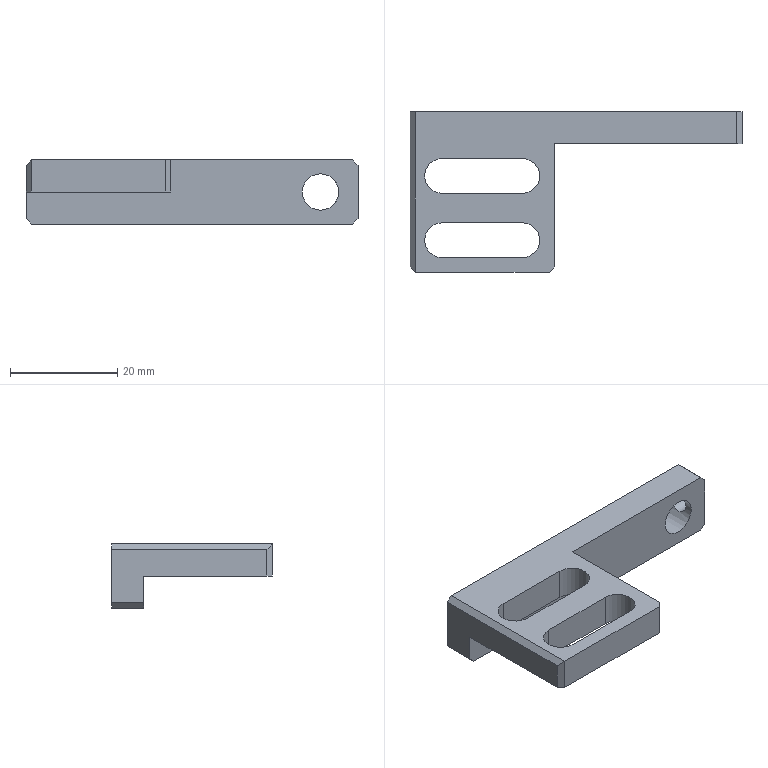NC program | NX | posted with a generic post | part box 62 x 30 x 12 mm
Lines 1 to 1127 of 2452:
N10 G17 G21 G94 G90
(FLOOR_WALL , TOOL : D80)
N12 T19 M6
N14 G54
N16 G17 G0 G90 X-79. Y0. S6500 M3
N18 G43 Z30. H19
N20 Z3.
N22 G94 G1 Z0. F1500.
N24 X-76.
N26 X76.
N28 X79.
N30 Z3.
N32 G0 Z30.
N34 M5
(ADAPTIVE_MILLING , TOOL : D10)
N36 T15 M6
N38 G54
N40 G17 G0 G90 X-43.696 Y9.051 S9500 M3
N42 G43 Z30. H15
N44 Z-9.
N46 G94 G1 Z-12. F1000.
N48 X-42.34 Y8.521 F3000.
N50 G3 X-41.05 Y9.051 R1.015
N52 X-40.406 Y12.21 R9.424
N54 X-40.205 Y17.805 R187.645
N56 G2 X-37.222 Y22.096 R6.12
N58 X-31.636 Y23.842 R13.446
N60 X-22.247 Y24.18 R89.73
N62 G1 X-20.347 Y24.185
N64 X-17.347 Y24.189
N66 X-10.147 Y24.19
N68 X33.353
N70 X33.453 Y24.188
N72 X33.553 Y24.183
N74 G2 X37.956 Y21.388 R5.941
N76 X39.823 Y15.744 R12.962
N78 X40.176 Y7.056 R79.199
N80 G1 X40.182 Y5.556
N82 X40.187 Y3.356
N84 X40.19 Y-0.444
N86 Y-17.344
N88 X40.189 Y-17.444
N90 X40.184 Y-17.544
N92 G2 X37.56 Y-21.836 R5.866
N94 X32.049 Y-23.779 R12.34
N96 X23.864 Y-24.17 R67.44
N98 G1 X22.564 Y-24.178
N100 X20.964 Y-24.184
N102 X18.464 Y-24.188
N104 X13.564 Y-24.19
N106 X-33.336
N108 X-33.436 Y-24.189
N110 G2 X-37.832 Y-21.568 R5.82
N112 X-39.764 Y-16.158 R12.207
N114 X-40.172 Y-7.474 R69.436
N116 X-40.159 Y6.625 R759.67
N118 G3 X-39.485 Y15.297 R155.91
N120 G2 X-35.334 Y21.202 R7.866
N122 X-28.936 Y23.024 R16.463
N124 X-19.346 Y23.367 R100.863
N126 G1 X-17.646 Y23.374
N128 X-15.246 Y23.378
N130 X-11.046 Y23.381
N132 X9.754 Y23.382
N134 X30.454
N136 X30.654 Y23.38
N138 G2 X36.983 Y19.6 R7.588
N140 X38.954 Y13.459 R15.207
N142 X39.366 Y3.573 R87.274
N144 G1 X39.373 Y1.873
N146 X39.378 Y-0.427
N148 X39.381 Y-4.227
N150 X39.382 Y-14.527
N152 X39.381 Y-14.627
N154 X39.376 Y-14.827
N156 G2 X35.623 Y-20.967 R7.581
N158 X29.584 Y-22.934 R14.985
N160 X20. Y-23.363 R80.802
N162 G1 X18.4 Y-23.371
N164 X16.4 Y-23.376
N166 X13.3 Y-23.38
N168 X6.2 Y-23.382
N170 X-30.5
N172 X-30.7 Y-23.38
N174 G2 X-36.954 Y-19.648 R7.559
N176 X-38.956 Y-13.414 R15.247
N178 X-39.361 Y-4.328 R81.183
N180 X-39.306 Y5.97 R217.252
N182 X-38.737 Y13.648 R271.341
N184 X-33.658 Y20.415 R9.134
N186 X-26.832 Y22.212 R18.952
N188 X-15.442 Y22.563 R126.701
N190 G1 X-13.242 Y22.568
N192 X-9.742 Y22.572
N194 X-1.242 Y22.573
N196 X28.158
N198 X28.358 Y22.571
N200 X28.558 Y22.567
N202 G2 X36.25 Y17.814 R8.78
N204 X38.166 Y11.129 R17.751
N206 X38.556 Y0.742 R103.678
N208 X38.545 Y-13.058 R767.731
N210 X33.726 Y-20.299 R8.807
N212 X27.028 Y-22.175 R18.02
N214 X16.939 Y-22.556 R103.246
N216 G1 X15.339 Y-22.563
N218 X13.039 Y-22.568
N220 X9.439 Y-22.572
N222 X0.139 Y-22.573
N224 X-28.161
N226 X-28.361 Y-22.571
N228 G2 X-36.299 Y-17.724 R8.819
N230 X-38.175 Y-11.027 R18.
N232 X-38.556 Y-0.938 R103.676
N234 X-38.023 Y11.943 R113.361
N236 X-35.561 Y17.211 R10.199
N238 X-32.473 Y19.87 R5.126
N240 X-23.965 Y21.514 R28.511
N242 X-11.069 Y21.759 R226.459
N244 G1 X-7.669 Y21.763
N246 X-0.269 Y21.764
N248 X26.131
N250 X26.331 Y21.763
N252 X26.531 Y21.76
N254 X26.731 Y21.755
N256 G2 X32.627 Y19.799 R9.712
N258 X34.648 Y18.552 R5.351
N260 X35.9 Y16.384 R5.818
N262 X37.518 Y7.868 R29.466
N264 X37.76 Y-5.528 R242.06
N266 X37.694 Y-11.726 R97.141
N268 X33.047 Y-19.035 R9.453
N270 X30.839 Y-20.166 R6.945
N272 X23.089 Y-21.543 R27.373
N274 X10.292 Y-21.76 R245.397
N276 G1 X6.292 Y-21.763
N278 X-5.208 Y-21.765
N280 X-26.108 Y-21.764
N282 X-26.308 Y-21.763
N284 X-26.508 Y-21.76
N286 X-26.708 Y-21.756
N288 G2 X-35.471 Y-16.282 R9.676
N290 X-37.357 Y-9.273 R19.838
N292 X-37.33 Y10.103 R115.32
N294 X-36.142 Y14.112 R13.218
N296 G3 X-36.096 Y15.034 R7.65
N298 G2 X-35.517 Y17.307 R5.644
N300 G1 X-35.375 Y17.605
N302 G2 X-33.486 Y19.443 R5.742
N304 X-30.566 Y20.113 R6.237
N306 X-19.894 Y20.847 R168.837
N308 X1.905 Y20.956 R945.884
N310 G1 X24.205
N312 X24.505 Y20.954
N314 X24.905 Y20.948
N316 X25.105 Y20.942
N318 X25.405 Y20.931
N320 G2 X29.506 Y20.11 R13.83
N322 X32.384 Y19.9 R13.094
N324 G1 X32.661 Y19.785
N326 G3 X33.089 Y21.901 R-1.1
N328 G1 X-30.959 Y22.3
N330 G3 X-32.064 Y21.205 R1.1
N332 X-30.966 Y20.1 R1.1
N334 G1 X29.634
N336 G2 X32.384 Y19.9 R11.507
N338 X35.443 Y17.486 R5.403
N340 G1 X35.9 Y16.384
N342 G2 X36.226 Y13.07 R33.493
N344 X36.93 Y-1.605 R135.551
N346 X36.899 Y-9.904 R191.65
N348 X36.115 Y-13.403 R12.201
N350 X35.9 Y-15.384 R13.073
N352 X34.582 Y-17.631 R5.988
N354 X33.024 Y-19.053 R11.464
N356 G3 X33.779 Y-20.836 R1.001
N358 G1 X34.128 Y-20.728 Z-11.982
N360 X34.465 Y-20.584 Z-11.963
N362 X35.636 Y-20.1 Z-11.9
N364 X36.391 Y-19.79
N366 X37.139 Y-19.466
N368 G3 X37.524 Y-19.053 R1.053
N370 G1 X38.027 Y-18.049
N372 X38.491 Y-17.027
N374 G3 X39.117 Y-15.003 R15.794
N376 X39.805 Y-10.496 R23.573
N378 X40.015 Y-5.102 R70.637
N380 G1 X39.997 Y12.616
N382 G3 X39.762 Y13.259 R1.033
N384 G1 X38.615 Y14.62
N386 X38.19 Y15.132 Z-11.933
N388 X37.747 Y15.628 Z-11.967
N390 G3 X37.135 Y15.865 Z-12. R1.04
N392 X36.1 Y14.866 R1.004
N394 G1 Y-13.534
N396 G2 X35.375 Y-16.605 R5.929
N398 X32.486 Y-19.443 R10.841
N400 X29.766 Y-20.112 R6.204
N402 X13.496 Y-20.934 R139.776
N404 G1 X11.796 Y-20.943
N406 X9.696 Y-20.949
N408 X6.596 Y-20.953
N410 X0.896 Y-20.955
N412 X-24.204 Y-20.956
N414 X-24.504 Y-20.954
N416 G2 X-30.723 Y-19.402 R11.387
N418 X-35.415 Y-13.116 R11.727
N420 X-36.743 Y-5.152 R29.65
N422 X-36.572 Y8.735 R95.286
N424 X-36.1 Y11.151 R40.097
N426 G1 Y14.351
N428 G3 X-37.762 Y15.1 R1.001
N430 X-38.109 Y14.501 Z-11.965 R1.29
N432 G1 X-38.548 Y13.279 Z-11.9
N434 X-39.262 Y11.276
N436 X-39.578 Y8.833
N438 X-39.876 Y6.387
N440 G3 X-40.05 Y-0.017 R43.844
N442 G1 X-39.733 Y-6.525
N444 G3 X-38.657 Y-13.017 R37.122
N446 X-36.945 Y-16.979 R15.29
N448 G1 X-35.739 Y-18.923
N450 G3 X-34.353 Y-20.457 R6.568
N452 G1 X-33.204 Y-21.353
N454 X-32.042 Y-22.234
N456 G3 X-30.162 Y-23.087 R5.915
N458 G1 X-28.952 Y-23.383
N460 X-27.731 Y-23.633
N462 G3 X-25.254 Y-23.843 R16.752
N464 G1 X-9.424 Y-23.948
N466 X-2.342 Y-23.975
N468 X27.716 Y-23.997
N470 G3 X28.361 Y-23.762 R1.033
N472 G1 X29.72 Y-22.615
N474 X30.232 Y-22.19 Z-11.933
N476 X30.728 Y-21.747 Z-11.967
N478 G3 X30.965 Y-21.135 Z-12. R1.04
N480 X29.966 Y-20.1 R1.004
N482 G1 X5.034
N484 X4.734 Y-20.106
N486 X3.835 Y-20.122
N488 X3.235 Y-20.128
N490 X2.235 Y-20.134
N492 X0.635 Y-20.14
N494 X-1.865 Y-20.144
N496 X-6.565 Y-20.147
N498 X-22.465
N500 G2 X-28.064 Y-19.298 R14.635
N502 X-34.067 Y-13.176 R11.214
N504 X-35.794 Y-5.502 R24.468
N506 X-35.84 Y7.384 R89.108
N508 X-36.1 Y9.034 R13.2
N510 G1 Y11.234
N512 G3 X-37.542 Y12.131 R1.002
N514 X-38.104 Y11.403 Z-11.953 R1.145
N516 G1 X-38.47 Y10.417 Z-11.9
N518 X-39.254 Y8.287
N520 X-39.282 Y8.052
N522 X-39.286 Y3.678
N524 X-39.268 Y-0.696
N526 G3 X-38.777 Y-6.914 R56.986
N528 G1 X-38.41 Y-9.51
N530 G3 X-35.769 Y-16.316 R18.713
N532 X-34.047 Y-18.757 R19.896
N534 X-32.59 Y-20.099 R9.254
N536 G1 X-31.685 Y-20.765
N538 X-30.752 Y-21.39
N540 G3 X-27.032 Y-22.706 R9.411
N542 X-20.82 Y-23.161 R50.522
N544 G1 X1.852 Y-23.282
N546 X2.035 Y-23.261
N548 X2.213 Y-23.217
N550 X4.065 Y-22.512
N552 X4.773 Y-22.248 Z-11.938
N554 X5.472 Y-21.962 Z-11.976
N556 X5.664 Y-21.812 Z-11.988
N558 X5.819 Y-21.625 Z-12.
N560 G3 X5.034 Y-20.1 R1.002
N562 G2 X2.24 Y-19.648 R50.604
N564 G3 X-6.451 Y-19.365 R85.897
N566 G2 X-22.65 Y-19.303 R846.646
N568 X-29.998 Y-16.571 R11.587
N570 X-34.017 Y-9.783 R13.902
N572 X-35.146 Y-1.177 R36.893
N574 X-35.121 Y5.821 R154.945
N576 G3 X-35.443 Y6.514 R1.939
N578 G1 X-35.9 Y7.616
N580 G3 X-37.056 Y8.206 R1.006
N582 X-37.807 Y7.491 Z-11.946 R1.106
N584 G1 X-38.196 Y6.66 Z-11.9
N586 X-39.041 Y4.832
N588 X-39.078 Y4.635
N590 X-39.082 Y4.434
N592 G3 X-38.256 Y-3.007 R212.114
N594 G1 X-37.921 Y-5.548
N596 X-37.566 Y-8.087
N598 G3 X-34.602 Y-15.694 R20.015
N600 X-32.623 Y-18.416 R29.81
N602 X-29.897 Y-20.547 R9.512
N604 X-25.171 Y-22.053 R14.626
N606 G1 X-24.178 Y-22.134
N608 X0.434 Y-23.082
N610 X0.666 Y-23.06
N612 X0.888 Y-22.992
N614 X2.627 Y-22.2
N616 X3.777 Y-21.664 Z-11.964
N618 G3 X4.199 Y-21.087 Z-12. R1.031
N620 X3.616 Y-19.9 R1.005
N622 X-1.124 Y-18.79 R12.613
N624 X-12.32 Y-18.569 R173.619
N626 G2 X-21.718 Y-18.474 R218.03
N628 X-32.202 Y-11.323 R11.783
N630 X-34.089 Y-3.485 R24.256
N632 X-34.341 Y4.207 R92.773
N634 G3 X-34.648 Y5.448 R2.107
N636 G1 X-35.318 Y6.321
N638 G3 X-36.621 Y6.572 R1.005
N640 X-37.127 Y5.668 Z-11.946 R1.107
N642 G1 X-37.253 Y4.758 Z-11.9
N644 X-37.419 Y3.592
N646 X-37.568 Y2.424
N648 X-37.554 Y-0.907
N650 G3 X-37.077 Y-5.028 R25.941
N652 G1 X-36.699 Y-6.927
N654 X-36.304 Y-8.822
N656 G3 X-34.588 Y-13.35 R18.176
N658 G1 X-34.106 Y-14.148
N660 X-33.581 Y-14.918
N662 X-32.845 Y-15.919
N664 X-32.065 Y-16.884
N666 G3 X-26.419 Y-20.556 R12.44
N668 X-22.768 Y-21.288 R18.174
N670 X-17.797 Y-21.722 R80.995
N672 G1 X-0.582 Y-22.661
N674 X-0.341 Y-22.641
N676 X-0.11 Y-22.571
N678 X1.597 Y-21.788
N680 X2.196 Y-21.519 Z-11.933
N682 X2.784 Y-21.227 Z-11.966
N684 G3 X3.178 Y-20.681 Z-12. R1.039
N686 X2.6 Y-19.479 R1.005
N688 X-0.981 Y-18.237 R7.957
N690 X-8.864 Y-17.81 R62.744
N692 G2 X-20.362 Y-17.677 R361.925
N694 X-27.846 Y-14.969 R12.565
N696 X-32.197 Y-8.041 R14.152
N698 X-33.435 Y0.947 R34.334
N700 G3 X-33.746 Y4.424 R15.66
N702 X-34.552 Y5.352 R1.764
N704 G1 X-34.622 Y5.423
N706 G3 X-35.804 Y5.596 R1.007
N708 X-36.332 Y4.785 Z-11.95 R1.037
N710 G1 X-36.499 Y3.806 Z-11.9
N712 X-36.858 Y1.693
N714 G3 X-36.784 Y-1.216 R20.537
N716 G1 X-36.627 Y-2.2
N718 X-35.716 Y-6.69
N720 G3 X-33.878 Y-11.94 R24.631
N722 X-31.975 Y-14.92 R17.789
N724 G1 X-31.005 Y-16.143
N726 X-30.014 Y-17.348
N728 G3 X-29.072 Y-18.147 R4.229
N730 X-25.681 Y-19.665 R11.329
N732 X-21.104 Y-20.564 R25.103
N734 G1 X-19.707 Y-20.692
N736 X-18.306 Y-20.78
N738 X-1.569 Y-21.503
N740 X0.65 Y-21.194
N742 X1.296 Y-21.109 Z-11.933
N744 X1.937 Y-20.997 Z-11.965
N746 G3 X2.476 Y-20.577 Z-12. R1.038
N748 X2.237 Y-19.253 R1.005
N750 X-1.366 Y-17.64 R7.137
N752 X-8.934 Y-17.05 R46.203
N754 G2 X-19.331 Y-16.865 R298.69
N756 X-27.054 Y-13.964 R12.902
N758 X-31.385 Y-6.904 R14.556
N760 X-32.548 Y0.691 R34.111
N762 G3 X-33.081 Y4.037 R12.519
N764 X-33.605 Y4.625 R1.254
N766 G1 X-34.16 Y5.051
N768 G3 X-35.269 Y5.124 R1.01
N770 X-35.766 Y4.384 Z-11.954 R1.049
N772 G1 X-36.005 Y3.332 Z-11.9
N774 X-36.223 Y2.384
N776 X-36.426 Y1.433
N778 X-36.41 Y1.154
N780 X-35.15 Y-5.094
N782 G3 X-32.833 Y-11.401 R26.03
N784 G1 X-32.295 Y-12.424
N786 X-31.713 Y-13.423
N788 G3 X-29.574 Y-15.898 R13.141
N790 X-25.379 Y-18.52 R12.096
N792 X-21.183 Y-19.628 R18.366
N794 G1 X-19.323 Y-19.841
N796 X-17.458 Y-19.996
N798 X-2.272 Y-20.956
N800 X-0.077 Y-20.65
N802 X0.574 Y-20.562 Z-11.933
N804 X1.222 Y-20.45 Z-11.966
N806 G3 X1.755 Y-20.04 Z-12. R1.039
N808 X1.523 Y-18.705 R1.005
N810 X-1.527 Y-17.098 R6.057
N812 X-8.77 Y-16.309 R34.863
N814 G2 X-18.266 Y-16.061 R306.262
N816 X-25.777 Y-13.381 R13.381
N818 X-30.447 Y-6.198 R14.425
N820 X-31.665 Y0.481 R36.713
N822 G3 X-32.444 Y3.775 R10.534
N824 X-33.486 Y4.557 R1.623
N826 G1 X-33.573 Y4.607
N828 G3 X-34.762 Y4.466 R1.007
N830 X-35.059 Y3.545 Z-11.95 R1.037
N832 G1 X-34.963 Y2.557 Z-11.9
N834 X-34.738 Y0.26
N836 X-34.361 Y-2.273
N838 X-33.963 Y-4.803
N840 G3 X-31.087 Y-11.847 R19.064
N842 X-28.732 Y-14.984 R31.932
N844 X-25.067 Y-17.484 R9.806
N846 X-20.281 Y-18.776 R17.825
N848 G1 X-17.807 Y-19.112
N850 X-15.326 Y-19.39
N852 X-2.74 Y-20.62
N854 X-2.468 Y-20.609
N856 X-0.511 Y-20.263
N858 X0.141 Y-20.152 Z-11.933
N860 X0.788 Y-20.018 Z-11.966
N862 G3 X1.303 Y-19.598 Z-12. R1.039
N864 X1.157 Y-18.37 R1.007
N866 X-2.25 Y-16.405 R6.304
N868 X-9.584 Y-15.542 R34.158
N870 G2 X-17.676 Y-15.224 R159.973
N872 X-25.918 Y-11.582 R13.155
N874 X-29.94 Y-3.989 R15.973
N876 X-31.058 Y1.599 R292.744
N878 G3 X-32.025 Y3.878 R5.344
N880 X-33.03 Y4.368 R3.956
N882 X-34.128 Y4.144 R1.01
N884 X-34.406 Y3.289 Z-11.954 R1.048
N886 G1 X-34.344 Y2.221 Z-11.9
N888 X-34.217 Y0.124
N890 X-32.783 Y-5.093
N892 G3 X-31.442 Y-8.922 R46.768
N894 X-29.784 Y-11.838 R12.939
N896 G1 X-29.133 Y-12.59
N898 X-27.463 Y-14.323
N900 G3 X-21.454 Y-17.573 R13.048
N902 X-17.775 Y-18.232 R34.803
N904 G1 X-3.376 Y-19.983
N906 X-3.079 Y-19.975
N908 X-1.143 Y-19.628
N910 X-0.492 Y-19.517 Z-11.933
N912 X0.154 Y-19.381 Z-11.966
N914 G3 X0.669 Y-18.959 Z-12. R1.039
N916 X0.521 Y-17.733 R1.007
N918 X-2.193 Y-15.928 R5.309
N920 X-8.686 Y-14.861 R25.457
N922 G2 X-16.674 Y-14.434 R223.663
N924 X-24.715 Y-11.013 R13.575
N926 X-28.829 Y-4.03 R15.59
N928 X-30.234 Y1.39 R621.178
N930 G3 X-31.438 Y3.777 R5.753
N932 X-32.384 Y4.1 R1.989
N934 X-33.34 Y3.851 R1.014
N936 X-33.641 Y3.024 Z-11.955 R1.05
N938 G1 X-33.629 Y1.933 Z-11.9
N940 X-33.608 Y0.083
N942 X-33.588 Y-0.083
N944 X-33.548 Y-0.247
N946 X-32.466 Y-3.244
N948 X-31.363 Y-6.234
N950 G3 X-28.85 Y-10.813 R23.751
N952 G1 X-28.079 Y-11.871
N954 X-27.271 Y-12.902
N956 G3 X-24.137 Y-15.318 R10.546
N958 X-21.389 Y-16.481 R19.145
N960 X-18.97 Y-17.036 R17.581
N962 X-14.027 Y-17.682 R55.575
N964 G1 X-4.113 Y-18.51
N966 X-1.856 Y-18.798
N968 X-1.208 Y-18.886 Z-11.933
N970 X-0.557 Y-18.949 Z-11.965
N972 G3 X0.07 Y-18.69 Z-12. R1.038
N974 X0.19 Y-17.341 R1.005
N976 X-2.579 Y-15.307 R5.28
N978 X-9.15 Y-14.116 R24.496
N980 G2 X-16.13 Y-13.603 R125.732
N982 X-24.41 Y-9.575 R13.462
N984 X-28.13 Y-2.794 R17.473
N986 G3 X-29.727 Y2.046 R54.57
N988 X-30.984 Y3.818 R4.115
N990 X-31.994 Y4.031 R3.165
N992 X-32.994 Y3.533 R1.01
N994 X-33.041 Y2.628 Z-11.953 R1.046
N996 G1 X-32.701 Y1.623 Z-11.9
N998 G2 X-31.462 Y-2.264 R63.673
N1000 G3 X-29.961 Y-6.495 R41.24
N1002 X-28.552 Y-9.129 R19.862
N1004 G1 X-27.914 Y-10.128
N1006 X-27.261 Y-11.118
N1008 G3 X-25.426 Y-12.957 R8.991
N1010 X-21.661 Y-15.134 R18.773
N1012 X-19.3 Y-15.903 R17.878
N1014 X-14.414 Y-16.841 R32.851
N1016 G1 X-4.568 Y-17.952
N1018 X-2.288 Y-18.242
N1020 X-1.637 Y-18.33 Z-11.933
N1022 X-0.984 Y-18.393 Z-11.966
N1024 G3 X-0.361 Y-18.138 Z-12. R1.039
N1026 X-0.236 Y-16.786 R1.005
N1028 X-2.724 Y-14.771 R4.838
N1030 X-8.956 Y-13.426 R21.46
N1032 G2 X-15.622 Y-12.769 R100.939
N1034 X-26.136 Y-4.895 R13.694
N1036 X-28.252 Y0.394 R62.965
N1038 G3 X-30.008 Y3.509 R9.065
N1040 X-31.034 Y3.904 R1.255
N1042 G1 X-31.332 Y3.944
N1044 G3 X-32.335 Y3.441 R1.01
N1046 X-32.378 Y2.54 Z-11.953 R1.047
N1048 G1 X-32.037 Y1.529 Z-11.9
N1050 G3 X-29.547 Y-4.875 R56.221
N1052 X-28.166 Y-7.52 R33.479
N1054 X-24.315 Y-12.143 R20.55
N1056 X-19.46 Y-14.819 R13.104
N1058 X-14.005 Y-16.107 R44.251
N1060 G1 X-4.687 Y-17.663
N1062 X-2.588 Y-17.795
N1064 X-1.925 Y-17.841 Z-11.933
N1066 X-1.262 Y-17.864 Z-11.966
N1068 G3 X-0.666 Y-17.582 Z-12. R1.04
N1070 X-0.443 Y-16.486 R1.01
N1072 X-2.241 Y-14.554 R3.68
N1074 X-7.662 Y-12.903 R15.539
N1076 G2 X-14.312 Y-12.089 R552.246
N1078 X-25.138 Y-4.422 R14.224
N1080 X-27.622 Y0.927 R104.496
N1082 G3 X-29.483 Y3.622 R7.9
N1084 X-30.136 Y3.9 R1.46
N1086 G1 X-30.836
N1088 G3 X-31.714 Y3.38 R1.011
N1090 X-31.745 Y2.442 Z-11.952 R1.133
N1092 G1 X-31.458 Y1.452 Z-11.9
N1094 X-30.886 Y-0.498
N1096 G3 X-25.53 Y-9.549 R141.743
N1098 X-23.62 Y-11.418 R7.988
N1100 X-19.253 Y-13.797 R21.184
N1102 X-16.281 Y-14.72 R30.006
N1104 G1 X-14.464 Y-15.162
N1106 X-4.943 Y-17.282
N1108 X-4.786 Y-17.304
N1110 X-2.758 Y-17.426
N1112 X-2.088 Y-17.472 Z-11.934
N1114 X-1.417 Y-17.494 Z-11.967
N1116 G3 X-0.831 Y-17.224 Z-12. R1.041
N1118 X-0.596 Y-16.117 R1.01
N1120 X-2.625 Y-13.871 R4.103
N1122 X-8.134 Y-12.158 R16.462
N1124 G2 X-14.354 Y-11.174 R105.789
N1126 X-24.079 Y-4.084 R14.71
N1128 X-26.906 Y1.207 R146.192
N1130 G3 X-28.962 Y3.751 R7.309
N1132 X-30.235 Y3.9 R2.567
N1134 X-31.132 Y3.343 R1.011
N1136 X-31.145 Y2.441 Z-11.954 R1.156
N1138 G1 X-30.853 Y1.41 Z-11.9
N1140 X-30.595 Y0.47
N1142 X-30.311 Y-0.464
N1144 X-30.235 Y-0.6
N1146 X-28.574 Y-3.098
N1148 X-26.895 Y-5.583
N1150 G3 X-23.543 Y-9.599 R35.771
N1152 X-18.379 Y-12.986 R15.585
N1154 X-14.235 Y-14.343 R42.531
N1156 G1 X-5.033 Y-16.842
N1158 X-2.955 Y-16.967
N1160 X-2.282 Y-17.011 Z-11.934
N1162 X-1.607 Y-17.032 Z-11.968
N1164 G3 X-1.027 Y-16.767 Z-12. R1.042
N1166 X-0.787 Y-15.655 R1.01
N1168 X-2.753 Y-13.32 R4.043
N1170 X-8.018 Y-11.502 R15.799
N1172 G2 X-14.098 Y-10.301 R77.085
N1174 X-23.177 Y-3.521 R15.598
N1176 X-26.168 Y1.447 R338.304
N1178 G3 X-28.208 Y3.753 R7.808
N1180 X-29.482 Y3.9 R2.59
N1182 X-30.377 Y3.346 R1.011
N1184 X-30.395 Y2.449 Z-11.954 R1.159
N1186 G1 X-30.113 Y1.41 Z-11.9
N1188 X-29.621 Y-0.366
N1190 X-29.482 Y-0.6
N1192 X-24.406 Y-6.945
N1194 G3 X-20.317 Y-10.746 R18.555
N1196 X-16.663 Y-12.608 R20.299
N1198 G1 X-15.258 Y-13.12
N1200 X-5.282 Y-16.416
N1202 X-5.113 Y-16.452
N1204 X-4.94 Y-16.467
N1206 X-3.195 Y-16.418
N1208 X-1.759 Y-16.368 Z-11.972
N1210 G3 X-1.259 Y-16.127 Z-12. R1.055
N1212 X-0.935 Y-15.252 R1.015
N1214 X-2.176 Y-13.27 R3.067
N1216 X-6.572 Y-11.188 R11.698
N1218 X-12.514 Y-9.814 R753.007
N1220 G2 X-22.293 Y-2.977 R16.762
N1222 G3 X-25.653 Y1.992 R415.359
N1224 X-27.496 Y3.801 R6.75
N1226 X-28.782 Y3.9 R3.469
N1228 X-29.746 Y3.164 R1.007
N1230 X-29.487 Y2.167 Z-11.946 R1.11
N1232 G1 X-28.948 Y1.414 Z-11.9
N1234 X-27.617 Y-0.447
N1236 X-24.766 Y-4.704
N1238 G3 X-22.033 Y-7.938 R23.298
N1240 X-18.852 Y-10.31 R18.351
N1242 X-13.417 Y-12.751 R22.588
N1244 G1 X-5.419 Y-15.067
N1246 X-3.39 Y-15.753
N1248 X-2.756 Y-15.973 Z-11.934
N1250 X-2.114 Y-16.171 Z-11.967
N1252 G3 X-1.478 Y-16.064 Z-12. R1.041
N1254 X-0.961 Y-15.053 R1.01
N1256 X-2.226 Y-12.755 R3.263
N1258 X-6.848 Y-10.462 R12.171
N1260 G2 X-12.82 Y-8.801 R126.102
N1262 X-21.451 Y-2.417 R18.169
N1264 G3 X-24.922 Y2.229 R197.188
N1266 X-26.696 Y3.822 R6.517
N1268 X-27.922 Y3.9 R3.927
N1270 X-28.886 Y3.164 R1.007
N1272 X-28.628 Y2.168 Z-11.946 R1.11
N1274 G1 X-28.089 Y1.414 Z-11.9
N1276 X-26.757 Y-0.447
N1278 X-25.047 Y-2.733
N1280 X-23.321 Y-5.008
N1282 G3 X-16.108 Y-10.636 R19.965
N1284 X-11.483 Y-12.49 R54.934
N1286 G1 X-7.477 Y-13.883
N1288 X-3.463 Y-15.255
N1290 X-2.826 Y-15.476 Z-11.934
N1292 X-2.181 Y-15.675 Z-11.968
N1294 G3 X-1.551 Y-15.572 Z-12. R1.042
N1296 X-1.027 Y-14.558 R1.01
N1298 X-2.408 Y-12.1 R3.534
N1300 X-6.912 Y-9.781 R12.901
N1302 G2 X-12.705 Y-7.879 R80.149
N1304 X-20.788 Y-1.679 R20.231
N1306 G3 X-24.486 Y2.786 R75.37
N1308 X-25.913 Y3.86 R4.408
N1310 X-27.026 Y3.9 R8.188
N1312 X-27.99 Y3.165 R1.007
N1314 X-27.732 Y2.168 Z-11.946 R1.11
N1316 G1 X-27.193 Y1.414 Z-11.9
N1318 X-25.861 Y-0.447
N1320 G3 X-22.835 Y-4.013 R72.245
N1322 G1 X-21.821 Y-5.075
N1324 X-20.791 Y-6.122
N1326 G3 X-15.266 Y-9.904 R21.503
N1328 X-10.155 Y-12.228 R113.987
N1330 G1 X-5.509 Y-14.188
N1332 X-3.521 Y-14.858
N1334 X-2.88 Y-15.079 Z-11.934
N1336 X-2.233 Y-15.278 Z-11.968
N1338 G3 X-1.607 Y-15.178 Z-12. R1.042
N1340 X-1.079 Y-14.161 R1.01
N1342 X-2.268 Y-11.719 R3.373
N1344 X-6.659 Y-9.198 R12.506
N1346 G2 X-12.543 Y-6.955 R71.678
N1348 X-20.114 Y-1.009 R22.877
N1350 G3 X-23.88 Y3.13 R49.551
N1352 X-25.188 Y3.9 R2.633
N1354 G1 X-26.188
N1356 G3 X-27.284 Y2.89 R1.106
N1358 X-26.738 Y1.843 Z-11.938 R1.124
N1360 G1 X-26.118 Y1.412 Z-11.9
N1362 X-3.597 Y-14.234
N1364 X-3.142 Y-14.555 Z-11.928
N1366 X-2.675 Y-14.858 Z-11.956
N1368 G3 X-1.813 Y-14.895 Z-12. R1.128
N1370 X-1.1 Y-13.866 R1.108
N1372 X-2.118 Y-11.35 R3.255
N1374 X-6.202 Y-8.707 R11.843
N1376 G2 X-12.167 Y-6.131 R86.348
N1378 X-19.494 Y-0.325 R26.4
N1380 G3 X-23.153 Y3.363 R37.963
N1382 X-24.207 Y3.9 R2.182
N1384 G1 X-25.207
N1386 G3 X-26.303 Y2.897 R1.106
N1388 X-25.762 Y1.846 Z-11.938 R1.124
N1390 G1 X-25.145 Y1.412 Z-11.9
N1392 X-3.612 Y-13.718
N1394 X-3.153 Y-14.044 Z-11.928
N1396 X-2.682 Y-14.354 Z-11.956
N1398 G3 X-1.834 Y-14.403 Z-12. R1.128
N1400 X-1.1 Y-13.366 R1.108
N1402 X-2.157 Y-10.757 R3.436
N1404 X-6.275 Y-7.979 R12.847
N1406 G2 X-12.546 Y-4.878 R64.102
N1408 X-18.865 Y0.311 R32.009
N1410 G3 X-22.304 Y3.507 R31.166
N1412 X-23.159 Y3.9 R1.919
N1414 G1 X-24.259
N1416 G3 X-25.354 Y2.903 R1.106
N1418 X-24.819 Y1.849 Z-11.938 R1.124
N1420 G1 X-24.204 Y1.412 Z-11.9
N1422 X-3.612 Y-13.212
N1424 X-3.155 Y-13.54 Z-11.928
N1426 X-2.687 Y-13.852 Z-11.956
N1428 G3 X-1.837 Y-13.904 Z-12. R1.128
N1430 X-1.1 Y-12.866 R1.108
N1432 X-2.115 Y-10.235 R3.552
N1434 X-5.967 Y-7.418 R13.085
N1436 G2 X-12.454 Y-3.866 R72.139
N1438 X-18.883 Y1.52 R45.77
N1440 G3 X-21.761 Y3.826 R14.344
N1442 X-23.176 Y3.9 R4.927
N1444 X-24.27 Y2.913 R1.106
N1446 X-23.744 Y1.853 Z-11.938 R1.124
N1448 G1 X-23.133 Y1.412 Z-11.9
N1450 X-3.612 Y-12.702
N1452 X-3.159 Y-13.033 Z-11.928
N1454 X-2.695 Y-13.348 Z-11.956
N1456 G3 X-1.843 Y-13.406 Z-12. R1.128
N1458 X-1.1 Y-12.366 R1.108
N1460 X-2.188 Y-9.556 R3.772
N1462 X-6.252 Y-6.515 R15.26
N1464 G2 X-13.547 Y-1.978 R58.761
N1466 X-18.942 Y2.636 R138.257
N1468 G3 X-20.754 Y3.864 R7.221
N1470 X-22.152 Y3.9 R12.842
N1472 X-23.245 Y2.922 R1.106
N1474 X-22.727 Y1.858 Z-11.938 R1.124
N1476 G1 X-22.121 Y1.412 Z-11.9
N1478 X-3.612 Y-12.193
N1480 X-3.163 Y-12.527 Z-11.928
N1482 X-2.702 Y-12.844 Z-11.956
N1484 G3 X-1.848 Y-12.908 Z-12. R1.128
N1486 X-1.1 Y-11.866 R1.108
N1488 X-2.184 Y-8.949 R3.922
N1490 X-5.991 Y-5.897 R15.848
N1492 G2 X-13.943 Y-0.535 R69.105
N1494 G3 X-18.739 Y3.392 R108.416
N1496 X-19.803 Y3.9 R2.441
N1498 G1 X-21.003
N1500 G3 X-22.095 Y2.931 R1.106
N1502 X-21.586 Y1.863 Z-11.938 R1.124
N1504 G1 X-20.984 Y1.412 Z-11.9
N1506 X-3.612 Y-11.583
N1508 X-3.167 Y-11.92 Z-11.928
N1510 X-2.71 Y-12.24 Z-11.956
N1512 G3 X-1.853 Y-12.309 Z-12. R1.128
N1514 X-1.1 Y-11.266 R1.108
N1516 X-2.102 Y-8.415 R3.958
N1518 X-6.048 Y-5.06 R16.956
N1520 G2 X-16.267 Y2.463 R96.04
N1522 G3 X-18.339 Y3.849 R11.209
N1524 X-19.892 Y3.9 R8.014
N1526 X-20.983 Y2.941 R1.106
N1528 X-20.483 Y1.868 Z-11.938 R1.124
N1530 G1 X-19.885 Y1.412 Z-11.9
N1532 X-3.612 Y-10.973
N1534 X-3.171 Y-11.313 Z-11.928
N1536 X-2.717 Y-11.636 Z-11.956
N1538 G3 X-1.859 Y-11.711 Z-12. R1.128
N1540 X-1.1 Y-10.666 R1.108
N1542 X-2.132 Y-7.72 R4.161
N1544 X-6.158 Y-4.151 R18.783
N1546 G2 X-15.602 Y2.92 R206.231
N1548 G3 X-17.228 Y3.882 R5.735
N1550 G1 X-17.327 Y3.898
N1552 X-17.346 Y3.9
N1554 X-18.646
N1556 G3 X-19.735 Y2.955 R1.106
N1558 X-19.25 Y1.876 Z-11.938 R1.124
N1560 G1 X-18.657 Y1.412 Z-11.9
N1562 X-3.612 Y-10.358
N1564 X-3.177 Y-10.702 Z-11.928
N1566 X-2.729 Y-11.03 Z-11.956
N1568 G3 X-1.867 Y-11.114 Z-12. R1.127
N1570 X-1.1 Y-10.066 R1.108
N1572 X-2.142 Y-7.017 R4.367
N1574 X-6.001 Y-3.409 R19.739
N1576 G1 X-6.479 Y-3.046
N1578 X-6.958 Y-2.685
N1580 X-7.759 Y-2.086
N1582 X-8.319 Y-1.666
N1584 X-8.8 Y-1.307
N1586 X-9.438 Y-0.825
N1588 X-10.074 Y-0.34
N1590 X-10.709 Y0.148
N1592 X-11.341 Y0.639
N1594 X-12.208 Y1.315
N1596 X-13.078 Y1.988
N1598 X-13.396 Y2.231
N1600 X-13.715 Y2.473
N1602 X-14.117 Y2.77
N1604 X-14.279 Y2.887
N1606 X-14.523 Y3.061
N1608 G3 X-15.997 Y3.888 R4.83
N1610 G1 X-16.096 Y3.9
N1612 X-17.396
N1614 G3 X-18.482 Y2.971 R1.106
N1616 X-18.013 Y1.885 Z-11.938 R1.124
N1618 G1 X-17.427 Y1.412 Z-11.9
N1620 X-3.611 Y-9.74
N1622 X-3.184 Y-10.089 Z-11.928
N1624 X-2.743 Y-10.422 Z-11.955
N1626 G3 X-1.878 Y-10.517 Z-12. R1.127
N1628 X-1.1 Y-9.466 R1.108
N1630 X-2.078 Y-6.391 R4.496
N1632 X-5.828 Y-2.669 R19.723
N1634 X-13.596 Y3.303 R190.392
N1636 X-14.819 Y3.9 R3.066
N1638 G1 X-16.119
N1640 G3 X-17.203 Y2.986 R1.106
N1642 X-16.75 Y1.894 Z-11.938 R1.124
N1644 G1 X-16.17 Y1.412 Z-11.9
N1646 X-3.611 Y-9.023
N1648 X-3.19 Y-9.377 Z-11.928
N1650 X-2.756 Y-9.715 Z-11.955
N1652 G3 X-1.888 Y-9.82 Z-12. R1.127
N1654 X-1.1 Y-8.766 R1.108
N1656 X-2.113 Y-5.596 R4.731
N1658 X-6.253 Y-1.417 R22.419
N1660 X-12.752 Y3.575 R72.725
N1662 X-13.545 Y3.9 R2.214
N1664 G1 X-14.845
N1666 G3 X-15.925 Y3.006 R1.106
N1668 X-15.494 Y1.907 Z-11.938 R1.124
N1670 G1 X-14.923 Y1.412 Z-11.9
N1672 X-3.611 Y-8.398
N1674 X-3.2 Y-8.759 Z-11.927
N1676 X-2.775 Y-9.104 Z-11.955
N1678 G3 X-1.903 Y-9.225 Z-12. R1.127
N1680 X-1.1 Y-8.166 R1.108
N1682 X-2.126 Y-4.795 R5.027
N1684 X-6.42 Y-0.348 R23.985
N1686 X-11.651 Y3.666 R44.795
N1688 X-12.29 Y3.9 R2.049
N1690 G1 X-13.59
N1692 G3 X-14.668 Y3.02 R1.106
N1694 X-14.252 Y1.916 Z-11.938 R1.124
N1696 G1 X-13.687 Y1.412 Z-11.9
N1698 X-3.611 Y-7.581
N1700 X-3.206 Y-7.947 Z-11.927
N1702 X-2.787 Y-8.296 Z-11.955
N1704 G3 X-1.914 Y-8.428 Z-12. R1.127
N1706 X-1.1 Y-7.366 R1.108
N1708 X-2.127 Y-3.991 R5.18
N1710 X-6.423 Y0.592 R24.095
N1712 X-10.639 Y3.789 R27.583
N1714 G1 X-10.731 Y3.828
N1716 X-10.826 Y3.86
N1718 X-10.923 Y3.883
N1720 X-11.022 Y3.898
N1722 X-11.039 Y3.9
N1724 X-12.339
N1726 G3 X-13.413 Y3.04 R1.106
N1728 X-13.02 Y1.931 Z-11.938 R1.125
N1730 G1 X-12.464 Y1.412 Z-11.9
N1732 X-3.61 Y-6.854
N1734 X-3.216 Y-7.227 Z-11.927
N1736 X-2.807 Y-7.583 Z-11.954
N1738 G3 X-1.931 Y-7.732 Z-12. R1.127
N1740 X-1.1 Y-6.666 R1.107
N1742 X-2.163 Y-3.097 R5.48
N1744 X-7.03 Y2.041 R25.371
N1746 X-9.549 Y3.834 R14.137
N1748 X-11.041 Y3.9 R5.874
N1750 X-12.109 Y3.062 R1.107
N1752 X-11.742 Y1.947 Z-11.938 R1.125
N1754 G1 X-11.196 Y1.412 Z-11.9
N1756 X-3.61 Y-6.024
N1758 X-2.85 Y-6.753 Z-11.953
N1760 G3 X-1.951 Y-6.937 Z-12. R1.117
N1762 X-1.1 Y-5.866 R1.106
N1764 X-2.131 Y-2.283 R5.636
N1766 X-8.195 Y3.734 R21.83
N1768 X-8.698 Y3.9 R4.335
N1770 G1 X-9.898
N1772 G3 X-10.962 Y3.079 R1.107
N1774 X-10.617 Y1.962 Z-11.939 R1.125
N1776 G1 X-10.078 Y1.412 Z-11.9
N1778 X-3.609 Y-5.198
N1780 X-2.868 Y-5.94 Z-11.953
N1782 G3 X-1.969 Y-6.141 Z-12. R1.117
N1784 X-1.1 Y-5.066 R1.106
N1786 X-2.198 Y-1.299 R5.906
N1788 X-7.129 Y3.741 R17.519
N1790 G1 X-7.616 Y3.9
N1792 X-8.716
N1794 G3 X-9.774 Y3.102 R1.108
N1796 X-9.459 Y1.983 Z-11.939 R1.126
N1798 G1 X-8.932 Y1.412 Z-11.9
N1800 X-3.609 Y-4.361
N1802 X-2.893 Y-5.12 Z-11.952
N1804 G3 X-1.995 Y-5.346 Z-12. R1.117
N1806 X-1.1 Y-4.266 R1.106
N1808 X-2.203 Y-0.399 R6.03
N1810 X-6.174 Y3.77 R13.697
N1812 G1 X-6.264 Y3.813
N1814 X-6.358 Y3.848
N1816 X-6.454 Y3.874
N1818 X-6.552 Y3.893
N1820 X-6.618 Y3.9
N1822 X-7.618
N1824 G3 X-8.67 Y3.12 R1.108
N1826 X-8.379 Y2. Z-11.939 R1.127
N1828 G1 X-7.862 Y1.411 Z-11.9
N1830 X-3.608 Y-3.429
N1832 X-2.913 Y-4.204 Z-11.952
N1834 G3 X-2.018 Y-4.45 Z-12. R1.117
N1836 X-1.1 Y-3.366 R1.106
N1838 X-2.255 Y0.587 R6.127
N1840 X-5.25 Y3.767 R10.624
N1842 G1 X-5.34 Y3.81
N1844 X-5.434 Y3.846
N1846 X-5.53 Y3.873
N1848 X-5.628 Y3.892
N1850 X-5.702 Y3.9
N1852 X-6.702
N1854 G3 X-7.751 Y3.13 R1.108
N1856 X-7.474 Y2.01 Z-11.939 R1.127
N1858 G1 X-6.962 Y1.411 Z-11.9
N1860 X-3.608 Y-2.511
N1862 X-2.924 Y-3.294 Z-11.952
N1864 G3 X-2.031 Y-3.553 Z-12. R1.117
N1866 X-1.1 Y-2.466 R1.106
N1868 X-2.263 Y1.483 R6.07
N1870 X-4.453 Y3.783 R7.699
N1872 X-5.765 Y3.9 R3.16
N1874 X-6.617 Y2.104 R1.101
N1876 G1 X-3.052 Y-2.261
N1878 G3 X-1.1 Y-1.566 R1.101
N1880 X-2.541 Y2.682 R5.924
N1882 X-3.885 Y3.85 R3.584
N1884 X-4.937 Y3.9 R5.327
N1886 X-5.8 Y2.118 R1.101
N1888 G1 X-3.063 Y-1.347
N1890 G3 X-1.1 Y-0.666 R1.101
N1892 X-3.092 Y3.784 R4.918
N1894 X-4.203 Y3.9 R2.565
N1896 X-5.07 Y2.123 R1.101
N1898 G1 X-3.067 Y-0.442
N1900 G3 X-1.1 Y0.234 R1.101
N1902 X-2.462 Y3.721 R4.047
N1904 X-3.589 Y3.9 R1.96
N1906 X-4.453 Y2.12 R1.101
N1908 G1 X-3.065 Y0.354
N1910 G3 X-1.1 Y1.034 R1.101
N1912 X-1.919 Y3.614 R3.255
N1914 X-3.077 Y3.9 R1.538
N1916 X-3.926 Y2.101 R1.101
N1918 G1 X-3.436 Y1.495
N1920 X-2.924 Y0.906
N1922 G3 X-1.1 Y1.734 R1.101
N1924 X-1.614 Y3.603 R2.448
N1926 X-2.587 Y3.9 R1.267
N1928 X-3.433 Y2.097 R1.101
N1930 G1 X-3.183 Y1.795
N1932 X-2.921 Y1.503
N1934 G3 X-1.1 Y2.334 R1.101
N1936 X-1.487 Y3.639 R1.51
N1938 X-2.35 Y3.9 R1.277
N1940 X-2.535 Y1.603 R1.157
N1942 X-1.113 Y2.952 R1.214
N1944 X-1.977 Y3.877 R1.033
N1946 X-1.552 Y1.984 R-1.036
N1948 X-1.113 Y2.949 R1.013
N1950 X-3.047 Y3.205 R1.011
N1952 G1 X-3.797 Y1.4
N1954 Z-9.
N1956 G0 Z30.
(FLOOR_WALL_1 , TOOL : D10)
N1958 X36.964 Y-19.35
N1960 Z-2.9
N1962 G1 Z-5.9 F1000.
N1964 X32.721
N1966 X2.279 F3000.
N1968 X1.633 Y-18.704
N1970 X33.367
N1972 X34.013 Y-18.058
N1974 X0.987
N1976 X0.341 Y-17.412
N1978 X34.659
N1980 X35.304 Y-16.767
N1982 X-0.304
N1984 X-0.95 Y-16.121
N1986 X35.95
N1988 X36. Y-16.071
N1990 Y-15.475
N1992 X-1.
N1994 Y-14.829
N1996 X36.
N1998 Y-14.183
N2000 X-1.
N2002 Y-13.537
N2004 X36.
N2006 Y-12.892
N2008 X-1.
N2010 Y-12.246
N2012 X36.
N2014 Y-11.6
N2016 X-1.
N2018 Y-10.954
N2020 X36.
N2022 Y-10.308
N2024 X-1.
N2026 Y-9.663
N2028 X36.
N2030 Y-9.017
N2032 X-1.
N2034 Y-8.371
N2036 X36.
N2038 Y-7.725
N2040 X-1.
N2042 Y-7.079
N2044 X36.
N2046 Y-6.433
N2048 X-1.
N2050 Y-5.788
N2052 X36.
N2054 Y-5.142
N2056 X-1.
N2058 Y-4.496
N2060 X36.
N2062 Y-3.85
N2064 X-1.
N2066 Y-3.204
N2068 X36.
N2070 Y-2.558
N2072 X-1.
N2074 Y-1.913
N2076 X36.
N2078 Y-1.267
N2080 X-1.
N2082 Y-0.621
N2084 X36.
N2086 Y0.025
N2088 X-1.
N2090 Y0.671
N2092 X36.
N2094 Y1.317
N2096 X-1.
N2098 Y1.962
N2100 X36.
N2102 Y2.608
N2104 X-1.
N2106 Y3.254
N2108 X36.
N2110 Y3.9
N2112 X-1.
N2114 X-4.
N2116 Y0.9
N2118 Z-2.9
N2120 G0 Z30.
N2122 M5
(ZLEVEL_PROFILE_COPY_1_COPY , TOOL : D10JING)
N2124 T14 M6
N2126 G54
N2128 G17 G0 G90 X-33.28 Y20.55 S9500 M3
N2130 G43 Z30. H14
N2132 Z-9.
N2134 G94 G1 Z-12. F1000.
N2136 G3 X-31. Y20. R5.
N2138 G1 X31. F1200.
N2140 G2 X36. Y15. R5.
N2142 G1 Y-14.
N2144 G2 X34.536 Y-17.536 R5.
N2146 G1 X33.536 Y-18.536
N2148 G2 X30. Y-20. R5.
N2150 G1 X5.
N2152 G2 X1.464 Y-18.536 R5.
N2154 G1 X0.464 Y-17.536
N2156 G2 X-1. Y-14. R5.
N2158 G1 Y4.
N2160 X-31.
N2162 G2 X-36. Y9. R5.
N2164 G1 Y15.
N2166 G2 X-31. Y20. R5.
N2168 G3 X-30.134 Y20.5 R1.
N2170 G1 X-29.845 Y21.
N2172 Z-11.
N2174 G0 Z30.
(FLOOR_WALL_1_COPY , TOOL : D10JING)
N2176 X39. Y-14.999
N2178 Z-3.
N2180 G1 Z-6. F1000.
N2182 X36.
N2184 X-1. F1500.
N2186 Y-10.374
N2188 X36.
N2190 Y-5.75
N2192 X-1.
N2194 Y-1.125
N2196 X36.
N2198 Y3.5
N2200 X-1.
N2202 X-4.
N2204 Y1.
N2206 Z-3.
N2208 G0 Z30.
N2210 X39. Y4.
N2212 Z-3.
N2214 G1 Z-6. F1000.
N2216 X36.
N2218 X-1. F1500.
N2220 X-4.
N2222 Y1.
N2224 Z-3.
N2226 G0 Z30.
N2228 M5